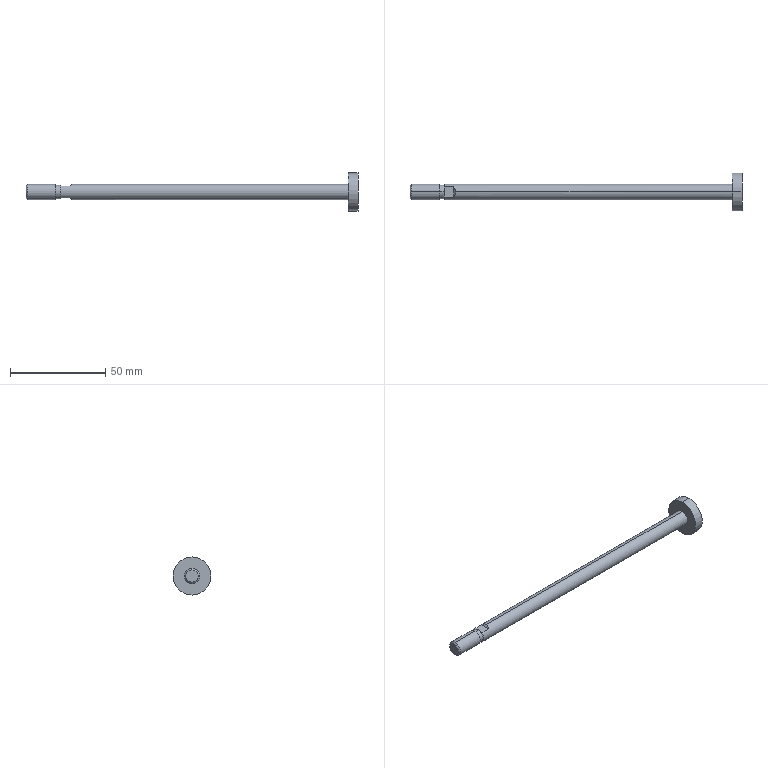Part | STEP file | _CM220-75SZ(0)_ROD | 1 solid | 22 faces | box 174.5 x 20 x 20 mm | volume 10018 mm3 | plane 12 | cylinder 8 | cone 2 | commonest cylinder face diameters 8 x4 7.1 x2 20 x2